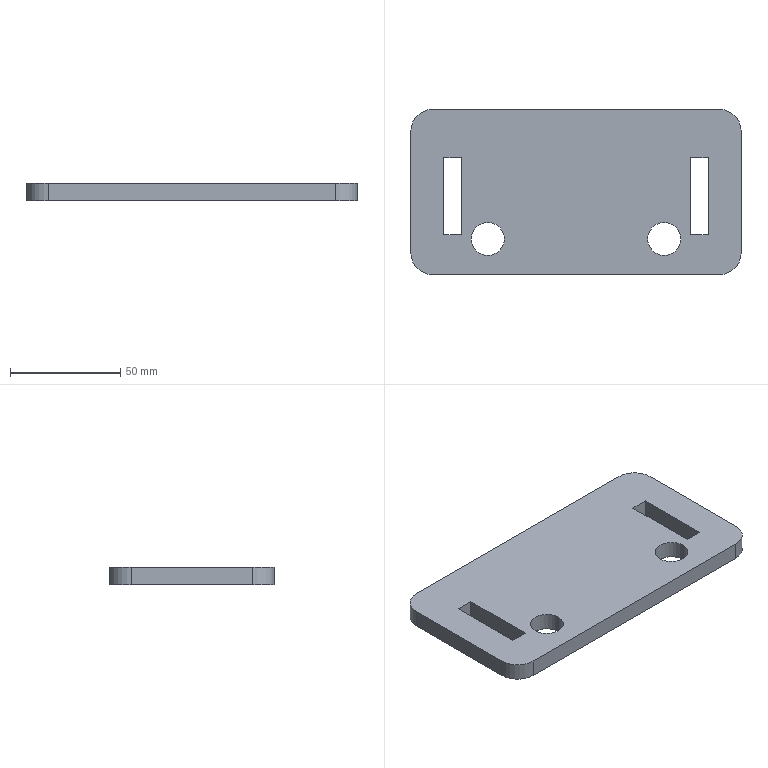Part | SolidWorks | features FlatPattern 1, SMBaseFlange 1, SheetMetal 1 | 1 solid | 22 faces | box 150 x 75 x 8 mm | volume 82006 mm3 | plane 14 | cylinder 8 | commonest cylinder face diameters 15 x4 20 x4
STEP:
#1=CARTESIAN_POINT('',(-47.5,148.277,8.));
#2=VERTEX_POINT('',#1);
#3=CARTESIAN_POINT('',(-32.5,148.277,8.));
#4=VERTEX_POINT('',#3);
#5=CARTESIAN_POINT('',(-40.,148.277,8.));
#6=DIRECTION('',(0.,0.,1.));
#7=DIRECTION('',(1.,0.,0.));
#8=AXIS2_PLACEMENT_3D('',#5,#6,#7);
#9=CIRCLE('',#8,7.5);
#10=EDGE_CURVE('',#2,#4,#9,.T.);
#11=ORIENTED_EDGE('',*,*,#10,.T.);
#12=CARTESIAN_POINT('',(-32.5,148.277,0.));
#13=VERTEX_POINT('',#12);
#14=CARTESIAN_POINT('',(-32.5,148.277,8.));
#15=DIRECTION('',(0.,0.,-1.));
#16=VECTOR('',#15,1000.);
#17=LINE('',#14,#16);
#18=EDGE_CURVE('',#4,#13,#17,.T.);
#19=ORIENTED_EDGE('',*,*,#18,.T.);
#20=CARTESIAN_POINT('',(-47.5,148.277,0.));
#21=VERTEX_POINT('',#20);
#22=CARTESIAN_POINT('',(-40.,148.277,0.));
#23=DIRECTION('',(0.,0.,1.));
#24=DIRECTION('',(1.,0.,0.));
#25=AXIS2_PLACEMENT_3D('',#22,#23,#24);
#26=CIRCLE('',#25,7.5);
#27=EDGE_CURVE('',#21,#13,#26,.T.);
#28=ORIENTED_EDGE('',*,*,#27,.F.);
#29=CARTESIAN_POINT('',(-47.5,148.277,8.));
#30=DIRECTION('',(0.,0.,-1.));
#31=VECTOR('',#30,1000.);
#32=LINE('',#29,#31);
#33=EDGE_CURVE('',#2,#21,#32,.T.);
#34=ORIENTED_EDGE('',*,*,#33,.F.);
#35=EDGE_LOOP('',(#11,#19,#28,#34));
#36=FACE_OUTER_BOUND('',#35,.T.);
#37=CARTESIAN_POINT('',(-40.,148.277,8.));
#38=DIRECTION('',(0.,0.,-1.));
#39=DIRECTION('',(-1.,0.,0.));
#40=AXIS2_PLACEMENT_3D('',#37,#38,#39);
#41=CYLINDRICAL_SURFACE('',#40,7.5);
#42=ADVANCED_FACE('',(#36),#41,.F.);
#43=CARTESIAN_POINT('',(32.5,148.277,8.));
#44=VERTEX_POINT('',#43);
#45=CARTESIAN_POINT('',(47.5,148.277,8.));
#46=VERTEX_POINT('',#45);
#47=CARTESIAN_POINT('',(40.,148.277,8.));
#48=DIRECTION('',(0.,0.,1.));
#49=DIRECTION('',(1.,0.,0.));
#50=AXIS2_PLACEMENT_3D('',#47,#48,#49);
#51=CIRCLE('',#50,7.5);
#52=EDGE_CURVE('',#44,#46,#51,.T.);
#53=ORIENTED_EDGE('',*,*,#52,.T.);
#54=CARTESIAN_POINT('',(47.5,148.277,0.));
#55=VERTEX_POINT('',#54);
#56=CARTESIAN_POINT('',(47.5,148.277,8.));
#57=DIRECTION('',(0.,0.,-1.));
#58=VECTOR('',#57,1000.);
#59=LINE('',#56,#58);
#60=EDGE_CURVE('',#46,#55,#59,.T.);
#61=ORIENTED_EDGE('',*,*,#60,.T.);
#62=CARTESIAN_POINT('',(32.5,148.277,0.));
#63=VERTEX_POINT('',#62);
#64=CARTESIAN_POINT('',(40.,148.277,0.));
#65=DIRECTION('',(0.,0.,1.));
#66=DIRECTION('',(1.,0.,0.));
#67=AXIS2_PLACEMENT_3D('',#64,#65,#66);
#68=CIRCLE('',#67,7.5);
#69=EDGE_CURVE('',#63,#55,#68,.T.);
#70=ORIENTED_EDGE('',*,*,#69,.F.);
#71=CARTESIAN_POINT('',(32.5,148.277,8.));
#72=DIRECTION('',(0.,0.,-1.));
#73=VECTOR('',#72,1000.);
#74=LINE('',#71,#73);
#75=EDGE_CURVE('',#44,#63,#74,.T.);
#76=ORIENTED_EDGE('',*,*,#75,.F.);
#77=EDGE_LOOP('',(#53,#61,#70,#76));
#78=FACE_OUTER_BOUND('',#77,.T.);
#79=CARTESIAN_POINT('',(40.,148.277,8.));
#80=DIRECTION('',(0.,0.,-1.));
#81=DIRECTION('',(-1.,0.,0.));
#82=AXIS2_PLACEMENT_3D('',#79,#80,#81);
#83=CYLINDRICAL_SURFACE('',#82,7.5);
#84=ADVANCED_FACE('',(#78),#83,.F.);
#85=ORIENTED_EDGE('',*,*,#52,.F.);
#86=CARTESIAN_POINT('',(40.,148.277,8.));
#87=DIRECTION('',(0.,0.,1.));
#88=DIRECTION('',(1.,0.,0.));
#89=AXIS2_PLACEMENT_3D('',#86,#87,#88);
#90=CIRCLE('',#89,7.5);
#91=EDGE_CURVE('',#46,#44,#90,.T.);
#92=ORIENTED_EDGE('',*,*,#91,.F.);
#93=EDGE_LOOP('',(#85,#92));
#94=FACE_BOUND('',#93,.T.);
#95=CARTESIAN_POINT('',(65.,132.079,8.));
#96=VERTEX_POINT('',#95);
#97=CARTESIAN_POINT('',(75.,142.079,8.));
#98=VERTEX_POINT('',#97);
#99=CARTESIAN_POINT('',(65.,142.079,8.));
#100=DIRECTION('',(0.,0.,1.));
#101=DIRECTION('',(1.,0.,0.));
#102=AXIS2_PLACEMENT_3D('',#99,#100,#101);
#103=CIRCLE('',#102,10.);
#104=EDGE_CURVE('',#96,#98,#103,.T.);
#105=ORIENTED_EDGE('',*,*,#104,.T.);
#106=CARTESIAN_POINT('',(75.,197.079,8.));
#107=VERTEX_POINT('',#106);
#108=CARTESIAN_POINT('',(75.,142.079,8.));
#109=DIRECTION('',(0.,1.,0.));
#110=VECTOR('',#109,1000.);
#111=LINE('',#108,#110);
#112=EDGE_CURVE('',#98,#107,#111,.T.);
#113=ORIENTED_EDGE('',*,*,#112,.T.);
#114=CARTESIAN_POINT('',(65.,207.079,8.));
#115=VERTEX_POINT('',#114);
#116=CARTESIAN_POINT('',(65.,197.079,8.));
#117=DIRECTION('',(0.,0.,1.));
#118=DIRECTION('',(1.,0.,0.));
#119=AXIS2_PLACEMENT_3D('',#116,#117,#118);
#120=CIRCLE('',#119,10.);
#121=EDGE_CURVE('',#107,#115,#120,.T.);
#122=ORIENTED_EDGE('',*,*,#121,.T.);
#123=CARTESIAN_POINT('',(-65.,207.079,8.));
#124=VERTEX_POINT('',#123);
#125=CARTESIAN_POINT('',(65.,207.079,8.));
#126=DIRECTION('',(-1.,0.,0.));
#127=VECTOR('',#126,1000.);
#128=LINE('',#125,#127);
#129=EDGE_CURVE('',#115,#124,#128,.T.);
#130=ORIENTED_EDGE('',*,*,#129,.T.);
#131=CARTESIAN_POINT('',(-75.,197.079,8.));
#132=VERTEX_POINT('',#131);
#133=CARTESIAN_POINT('',(-65.,197.079,8.));
#134=DIRECTION('',(0.,0.,1.));
#135=DIRECTION('',(1.,0.,0.));
#136=AXIS2_PLACEMENT_3D('',#133,#134,#135);
#137=CIRCLE('',#136,10.);
#138=EDGE_CURVE('',#124,#132,#137,.T.);
#139=ORIENTED_EDGE('',*,*,#138,.T.);
#140=CARTESIAN_POINT('',(-75.,142.079,8.));
#141=VERTEX_POINT('',#140);
#142=CARTESIAN_POINT('',(-75.,197.079,8.));
#143=DIRECTION('',(0.,-1.,0.));
#144=VECTOR('',#143,1000.);
#145=LINE('',#142,#144);
#146=EDGE_CURVE('',#132,#141,#145,.T.);
#147=ORIENTED_EDGE('',*,*,#146,.T.);
#148=CARTESIAN_POINT('',(-65.,132.079,8.));
#149=VERTEX_POINT('',#148);
#150=CARTESIAN_POINT('',(-65.,142.079,8.));
#151=DIRECTION('',(0.,0.,1.));
#152=DIRECTION('',(-1.,0.,0.));
#153=AXIS2_PLACEMENT_3D('',#150,#151,#152);
#154=CIRCLE('',#153,10.);
#155=EDGE_CURVE('',#141,#149,#154,.T.);
#156=ORIENTED_EDGE('',*,*,#155,.T.);
#157=CARTESIAN_POINT('',(-65.,132.079,8.));
#158=DIRECTION('',(1.,0.,0.));
#159=VECTOR('',#158,1000.);
#160=LINE('',#157,#159);
#161=EDGE_CURVE('',#149,#96,#160,.T.);
#162=ORIENTED_EDGE('',*,*,#161,.T.);
#163=EDGE_LOOP('',(#105,#113,#122,#130,#139,#147,#156,#162));
#164=FACE_OUTER_BOUND('',#163,.T.);
#165=ORIENTED_EDGE('',*,*,#10,.F.);
#166=CARTESIAN_POINT('',(-40.,148.277,8.));
#167=DIRECTION('',(0.,0.,1.));
#168=DIRECTION('',(1.,0.,0.));
#169=AXIS2_PLACEMENT_3D('',#166,#167,#168);
#170=CIRCLE('',#169,7.5);
#171=EDGE_CURVE('',#4,#2,#170,.T.);
#172=ORIENTED_EDGE('',*,*,#171,.F.);
#173=EDGE_LOOP('',(#165,#172));
#174=FACE_BOUND('',#173,.T.);
#175=CARTESIAN_POINT('',(60.,185.084,8.));
#176=VERTEX_POINT('',#175);
#177=CARTESIAN_POINT('',(52.,185.084,8.));
#178=VERTEX_POINT('',#177);
#179=CARTESIAN_POINT('',(60.,185.084,8.));
#180=DIRECTION('',(-1.,0.,0.));
#181=VECTOR('',#180,1000.);
#182=LINE('',#179,#181);
#183=EDGE_CURVE('',#176,#178,#182,.T.);
#184=ORIENTED_EDGE('',*,*,#183,.F.);
#185=CARTESIAN_POINT('',(60.,150.084,8.));
#186=VERTEX_POINT('',#185);
#187=CARTESIAN_POINT('',(60.,185.084,8.));
#188=DIRECTION('',(0.,1.,0.));
#189=VECTOR('',#188,1000.);
#190=LINE('',#187,#189);
#191=EDGE_CURVE('',#186,#176,#190,.T.);
#192=ORIENTED_EDGE('',*,*,#191,.F.);
#193=CARTESIAN_POINT('',(52.,150.084,8.));
#194=VERTEX_POINT('',#193);
#195=CARTESIAN_POINT('',(60.,150.084,8.));
#196=DIRECTION('',(1.,0.,0.));
#197=VECTOR('',#196,1000.);
#198=LINE('',#195,#197);
#199=EDGE_CURVE('',#194,#186,#198,.T.);
#200=ORIENTED_EDGE('',*,*,#199,.F.);
#201=CARTESIAN_POINT('',(52.,185.084,8.));
#202=DIRECTION('',(0.,-1.,0.));
#203=VECTOR('',#202,1000.);
#204=LINE('',#201,#203);
#205=EDGE_CURVE('',#178,#194,#204,.T.);
#206=ORIENTED_EDGE('',*,*,#205,.F.);
#207=EDGE_LOOP('',(#184,#192,#200,#206));
#208=FACE_BOUND('',#207,.T.);
#209=CARTESIAN_POINT('',(-52.,185.084,8.));
#210=VERTEX_POINT('',#209);
#211=CARTESIAN_POINT('',(-60.,185.084,8.));
#212=VERTEX_POINT('',#211);
#213=CARTESIAN_POINT('',(-52.,185.084,8.));
#214=DIRECTION('',(-1.,0.,0.));
#215=VECTOR('',#214,1000.);
#216=LINE('',#213,#215);
#217=EDGE_CURVE('',#210,#212,#216,.T.);
#218=ORIENTED_EDGE('',*,*,#217,.F.);
#219=CARTESIAN_POINT('',(-52.,150.084,8.));
#220=VERTEX_POINT('',#219);
#221=CARTESIAN_POINT('',(-52.,185.084,8.));
#222=DIRECTION('',(0.,1.,0.));
#223=VECTOR('',#222,1000.);
#224=LINE('',#221,#223);
#225=EDGE_CURVE('',#220,#210,#224,.T.);
#226=ORIENTED_EDGE('',*,*,#225,.F.);
#227=CARTESIAN_POINT('',(-60.,150.084,8.));
#228=VERTEX_POINT('',#227);
#229=CARTESIAN_POINT('',(-52.,150.084,8.));
#230=DIRECTION('',(1.,0.,0.));
#231=VECTOR('',#230,1000.);
#232=LINE('',#229,#231);
#233=EDGE_CURVE('',#228,#220,#232,.T.);
#234=ORIENTED_EDGE('',*,*,#233,.F.);
#235=CARTESIAN_POINT('',(-60.,185.084,8.));
#236=DIRECTION('',(0.,-1.,0.));
#237=VECTOR('',#236,1000.);
#238=LINE('',#235,#237);
#239=EDGE_CURVE('',#212,#228,#238,.T.);
#240=ORIENTED_EDGE('',*,*,#239,.F.);
#241=EDGE_LOOP('',(#218,#226,#234,#240));
#242=FACE_BOUND('',#241,.T.);
#243=CARTESIAN_POINT('',(65.,142.079,8.));
#244=DIRECTION('',(0.,0.,1.));
#245=DIRECTION('',(1.,0.,0.));
#246=AXIS2_PLACEMENT_3D('',#243,#244,#245);
#247=PLANE('',#246);
#248=ADVANCED_FACE('',(#94,#164,#174,#208,#242),#247,.T.);
#249=CARTESIAN_POINT('',(60.,150.084,0.));
#250=VERTEX_POINT('',#249);
#251=CARTESIAN_POINT('',(60.,185.084,0.));
#252=VERTEX_POINT('',#251);
#253=CARTESIAN_POINT('',(60.,185.084,0.));
#254=DIRECTION('',(0.,1.,0.));
#255=VECTOR('',#254,1000.);
#256=LINE('',#253,#255);
#257=EDGE_CURVE('',#250,#252,#256,.T.);
#258=ORIENTED_EDGE('',*,*,#257,.T.);
#259=CARTESIAN_POINT('',(52.,185.084,0.));
#260=VERTEX_POINT('',#259);
#261=CARTESIAN_POINT('',(60.,185.084,0.));
#262=DIRECTION('',(-1.,0.,0.));
#263=VECTOR('',#262,1000.);
#264=LINE('',#261,#263);
#265=EDGE_CURVE('',#252,#260,#264,.T.);
#266=ORIENTED_EDGE('',*,*,#265,.T.);
#267=CARTESIAN_POINT('',(52.,150.084,0.));
#268=VERTEX_POINT('',#267);
#269=CARTESIAN_POINT('',(52.,185.084,0.));
#270=DIRECTION('',(0.,-1.,0.));
#271=VECTOR('',#270,1000.);
#272=LINE('',#269,#271);
#273=EDGE_CURVE('',#260,#268,#272,.T.);
#274=ORIENTED_EDGE('',*,*,#273,.T.);
#275=CARTESIAN_POINT('',(60.,150.084,0.));
#276=DIRECTION('',(1.,0.,0.));
#277=VECTOR('',#276,1000.);
#278=LINE('',#275,#277);
#279=EDGE_CURVE('',#268,#250,#278,.T.);
#280=ORIENTED_EDGE('',*,*,#279,.T.);
#281=EDGE_LOOP('',(#258,#266,#274,#280));
#282=FACE_BOUND('',#281,.T.);
#283=CARTESIAN_POINT('',(65.,132.079,0.));
#284=VERTEX_POINT('',#283);
#285=CARTESIAN_POINT('',(75.,142.079,0.));
#286=VERTEX_POINT('',#285);
#287=CARTESIAN_POINT('',(65.,142.079,0.));
#288=DIRECTION('',(0.,0.,1.));
#289=DIRECTION('',(1.,0.,0.));
#290=AXIS2_PLACEMENT_3D('',#287,#288,#289);
#291=CIRCLE('',#290,10.);
#292=EDGE_CURVE('',#284,#286,#291,.T.);
#293=ORIENTED_EDGE('',*,*,#292,.F.);
#294=CARTESIAN_POINT('',(-65.,132.079,0.));
#295=VERTEX_POINT('',#294);
#296=CARTESIAN_POINT('',(-65.,132.079,0.));
#297=DIRECTION('',(1.,0.,0.));
#298=VECTOR('',#297,1000.);
#299=LINE('',#296,#298);
#300=EDGE_CURVE('',#295,#284,#299,.T.);
#301=ORIENTED_EDGE('',*,*,#300,.F.);
#302=CARTESIAN_POINT('',(-75.,142.079,0.));
#303=VERTEX_POINT('',#302);
#304=CARTESIAN_POINT('',(-65.,142.079,0.));
#305=DIRECTION('',(0.,0.,1.));
#306=DIRECTION('',(-1.,0.,0.));
#307=AXIS2_PLACEMENT_3D('',#304,#305,#306);
#308=CIRCLE('',#307,10.);
#309=EDGE_CURVE('',#303,#295,#308,.T.);
#310=ORIENTED_EDGE('',*,*,#309,.F.);
#311=CARTESIAN_POINT('',(-75.,197.079,0.));
#312=VERTEX_POINT('',#311);
#313=CARTESIAN_POINT('',(-75.,197.079,0.));
#314=DIRECTION('',(0.,-1.,0.));
#315=VECTOR('',#314,1000.);
#316=LINE('',#313,#315);
#317=EDGE_CURVE('',#312,#303,#316,.T.);
#318=ORIENTED_EDGE('',*,*,#317,.F.);
#319=CARTESIAN_POINT('',(-65.,207.079,0.));
#320=VERTEX_POINT('',#319);
#321=CARTESIAN_POINT('',(-65.,197.079,0.));
#322=DIRECTION('',(0.,0.,1.));
#323=DIRECTION('',(1.,0.,0.));
#324=AXIS2_PLACEMENT_3D('',#321,#322,#323);
#325=CIRCLE('',#324,10.);
#326=EDGE_CURVE('',#320,#312,#325,.T.);
#327=ORIENTED_EDGE('',*,*,#326,.F.);
#328=CARTESIAN_POINT('',(65.,207.079,0.));
#329=VERTEX_POINT('',#328);
#330=CARTESIAN_POINT('',(65.,207.079,0.));
#331=DIRECTION('',(-1.,0.,0.));
#332=VECTOR('',#331,1000.);
#333=LINE('',#330,#332);
#334=EDGE_CURVE('',#329,#320,#333,.T.);
#335=ORIENTED_EDGE('',*,*,#334,.F.);
#336=CARTESIAN_POINT('',(75.,197.079,0.));
#337=VERTEX_POINT('',#336);
#338=CARTESIAN_POINT('',(65.,197.079,0.));
#339=DIRECTION('',(0.,0.,1.));
#340=DIRECTION('',(1.,0.,0.));
#341=AXIS2_PLACEMENT_3D('',#338,#339,#340);
#342=CIRCLE('',#341,10.);
#343=EDGE_CURVE('',#337,#329,#342,.T.);
#344=ORIENTED_EDGE('',*,*,#343,.F.);
#345=CARTESIAN_POINT('',(75.,142.079,0.));
#346=DIRECTION('',(0.,1.,0.));
#347=VECTOR('',#346,1000.);
#348=LINE('',#345,#347);
#349=EDGE_CURVE('',#286,#337,#348,.T.);
#350=ORIENTED_EDGE('',*,*,#349,.F.);
#351=EDGE_LOOP('',(#293,#301,#310,#318,#327,#335,#344,#350));
#352=FACE_OUTER_BOUND('',#351,.T.);
#353=ORIENTED_EDGE('',*,*,#69,.T.);
#354=CARTESIAN_POINT('',(40.,148.277,0.));
#355=DIRECTION('',(0.,0.,1.));
#356=DIRECTION('',(1.,0.,0.));
#357=AXIS2_PLACEMENT_3D('',#354,#355,#356);
#358=CIRCLE('',#357,7.5);
#359=EDGE_CURVE('',#55,#63,#358,.T.);
#360=ORIENTED_EDGE('',*,*,#359,.T.);
#361=EDGE_LOOP('',(#353,#360));
#362=FACE_BOUND('',#361,.T.);
#363=ORIENTED_EDGE('',*,*,#27,.T.);
#364=CARTESIAN_POINT('',(-40.,148.277,0.));
#365=DIRECTION('',(0.,0.,1.));
#366=DIRECTION('',(1.,0.,0.));
#367=AXIS2_PLACEMENT_3D('',#364,#365,#366);
#368=CIRCLE('',#367,7.5);
#369=EDGE_CURVE('',#13,#21,#368,.T.);
#370=ORIENTED_EDGE('',*,*,#369,.T.);
#371=EDGE_LOOP('',(#363,#370));
#372=FACE_BOUND('',#371,.T.);
#373=CARTESIAN_POINT('',(-52.,150.084,0.));
#374=VERTEX_POINT('',#373);
#375=CARTESIAN_POINT('',(-52.,185.084,0.));
#376=VERTEX_POINT('',#375);
#377=CARTESIAN_POINT('',(-52.,185.084,0.));
#378=DIRECTION('',(0.,1.,0.));
#379=VECTOR('',#378,1000.);
#380=LINE('',#377,#379);
#381=EDGE_CURVE('',#374,#376,#380,.T.);
#382=ORIENTED_EDGE('',*,*,#381,.T.);
#383=CARTESIAN_POINT('',(-60.,185.084,0.));
#384=VERTEX_POINT('',#383);
#385=CARTESIAN_POINT('',(-52.,185.084,0.));
#386=DIRECTION('',(-1.,0.,0.));
#387=VECTOR('',#386,1000.);
#388=LINE('',#385,#387);
#389=EDGE_CURVE('',#376,#384,#388,.T.);
#390=ORIENTED_EDGE('',*,*,#389,.T.);
#391=CARTESIAN_POINT('',(-60.,150.084,0.));
#392=VERTEX_POINT('',#391);
#393=CARTESIAN_POINT('',(-60.,185.084,0.));
#394=DIRECTION('',(0.,-1.,0.));
#395=VECTOR('',#394,1000.);
#396=LINE('',#393,#395);
#397=EDGE_CURVE('',#384,#392,#396,.T.);
#398=ORIENTED_EDGE('',*,*,#397,.T.);
#399=CARTESIAN_POINT('',(-52.,150.084,0.));
#400=DIRECTION('',(1.,0.,0.));
#401=VECTOR('',#400,1000.);
#402=LINE('',#399,#401);
#403=EDGE_CURVE('',#392,#374,#402,.T.);
#404=ORIENTED_EDGE('',*,*,#403,.T.);
#405=EDGE_LOOP('',(#382,#390,#398,#404));
#406=FACE_BOUND('',#405,.T.);
#407=CARTESIAN_POINT('',(65.,142.079,0.));
#408=DIRECTION('',(0.,0.,1.));
#409=DIRECTION('',(1.,0.,0.));
#410=AXIS2_PLACEMENT_3D('',#407,#408,#409);
#411=PLANE('',#410);
#412=ADVANCED_FACE('',(#282,#352,#362,#372,#406),#411,.F.);
#413=ORIENTED_EDGE('',*,*,#292,.T.);
#414=CARTESIAN_POINT('',(75.,142.079,8.));
#415=DIRECTION('',(0.,0.,-1.));
#416=VECTOR('',#415,1000.);
#417=LINE('',#414,#416);
#418=EDGE_CURVE('',#98,#286,#417,.T.);
#419=ORIENTED_EDGE('',*,*,#418,.F.);
#420=ORIENTED_EDGE('',*,*,#104,.F.);
#421=CARTESIAN_POINT('',(65.,132.079,8.));
#422=DIRECTION('',(0.,0.,-1.));
#423=VECTOR('',#422,1000.);
#424=LINE('',#421,#423);
#425=EDGE_CURVE('',#96,#284,#424,.T.);
#426=ORIENTED_EDGE('',*,*,#425,.T.);
#427=EDGE_LOOP('',(#413,#419,#420,#426));
#428=FACE_OUTER_BOUND('',#427,.T.);
#429=CARTESIAN_POINT('',(65.,142.079,8.));
#430=DIRECTION('',(0.,0.,-1.));
#431=DIRECTION('',(-1.,0.,0.));
#432=AXIS2_PLACEMENT_3D('',#429,#430,#431);
#433=CYLINDRICAL_SURFACE('',#432,10.);
#434=ADVANCED_FACE('',(#428),#433,.T.);
#435=ORIENTED_EDGE('',*,*,#349,.T.);
#436=CARTESIAN_POINT('',(75.,197.079,8.));
#437=DIRECTION('',(0.,0.,-1.));
#438=VECTOR('',#437,1000.);
#439=LINE('',#436,#438);
#440=EDGE_CURVE('',#107,#337,#439,.T.);
#441=ORIENTED_EDGE('',*,*,#440,.F.);
#442=ORIENTED_EDGE('',*,*,#112,.F.);
#443=ORIENTED_EDGE('',*,*,#418,.T.);
#444=EDGE_LOOP('',(#435,#441,#442,#443));
#445=FACE_OUTER_BOUND('',#444,.T.);
#446=CARTESIAN_POINT('',(75.,142.079,8.));
#447=DIRECTION('',(-1.,0.,0.));
#448=DIRECTION('',(0.,-1.,0.));
#449=AXIS2_PLACEMENT_3D('',#446,#447,#448);
#450=PLANE('',#449);
#451=ADVANCED_FACE('',(#445),#450,.F.);
#452=ORIENTED_EDGE('',*,*,#343,.T.);
#453=CARTESIAN_POINT('',(65.,207.079,8.));
#454=DIRECTION('',(0.,0.,-1.));
#455=VECTOR('',#454,1000.);
#456=LINE('',#453,#455);
#457=EDGE_CURVE('',#115,#329,#456,.T.);
#458=ORIENTED_EDGE('',*,*,#457,.F.);
#459=ORIENTED_EDGE('',*,*,#121,.F.);
#460=ORIENTED_EDGE('',*,*,#440,.T.);
#461=EDGE_LOOP('',(#452,#458,#459,#460));
#462=FACE_OUTER_BOUND('',#461,.T.);
#463=CARTESIAN_POINT('',(65.,197.079,8.));
#464=DIRECTION('',(0.,0.,-1.));
#465=DIRECTION('',(-1.,0.,0.));
#466=AXIS2_PLACEMENT_3D('',#463,#464,#465);
#467=CYLINDRICAL_SURFACE('',#466,10.);
#468=ADVANCED_FACE('',(#462),#467,.T.);
#469=ORIENTED_EDGE('',*,*,#334,.T.);
#470=CARTESIAN_POINT('',(-65.,207.079,8.));
#471=DIRECTION('',(0.,0.,-1.));
#472=VECTOR('',#471,1000.);
#473=LINE('',#470,#472);
#474=EDGE_CURVE('',#124,#320,#473,.T.);
#475=ORIENTED_EDGE('',*,*,#474,.F.);
#476=ORIENTED_EDGE('',*,*,#129,.F.);
#477=ORIENTED_EDGE('',*,*,#457,.T.);
#478=EDGE_LOOP('',(#469,#475,#476,#477));
#479=FACE_OUTER_BOUND('',#478,.T.);
#480=CARTESIAN_POINT('',(65.,207.079,8.));
#481=DIRECTION('',(0.,-1.,0.));
#482=DIRECTION('',(1.,0.,0.));
#483=AXIS2_PLACEMENT_3D('',#480,#481,#482);
#484=PLANE('',#483);
#485=ADVANCED_FACE('',(#479),#484,.F.);
#486=ORIENTED_EDGE('',*,*,#326,.T.);
#487=CARTESIAN_POINT('',(-75.,197.079,8.));
#488=DIRECTION('',(0.,0.,-1.));
#489=VECTOR('',#488,1000.);
#490=LINE('',#487,#489);
#491=EDGE_CURVE('',#132,#312,#490,.T.);
#492=ORIENTED_EDGE('',*,*,#491,.F.);
#493=ORIENTED_EDGE('',*,*,#138,.F.);
#494=ORIENTED_EDGE('',*,*,#474,.T.);
#495=EDGE_LOOP('',(#486,#492,#493,#494));
#496=FACE_OUTER_BOUND('',#495,.T.);
#497=CARTESIAN_POINT('',(-65.,197.079,8.));
#498=DIRECTION('',(0.,0.,-1.));
#499=DIRECTION('',(-1.,0.,0.));
#500=AXIS2_PLACEMENT_3D('',#497,#498,#499);
#501=CYLINDRICAL_SURFACE('',#500,10.);
#502=ADVANCED_FACE('',(#496),#501,.T.);
#503=ORIENTED_EDGE('',*,*,#317,.T.);
#504=CARTESIAN_POINT('',(-75.,142.079,8.));
#505=DIRECTION('',(0.,0.,-1.));
#506=VECTOR('',#505,1000.);
#507=LINE('',#504,#506);
#508=EDGE_CURVE('',#141,#303,#507,.T.);
#509=ORIENTED_EDGE('',*,*,#508,.F.);
#510=ORIENTED_EDGE('',*,*,#146,.F.);
#511=ORIENTED_EDGE('',*,*,#491,.T.);
#512=EDGE_LOOP('',(#503,#509,#510,#511));
#513=FACE_OUTER_BOUND('',#512,.T.);
#514=CARTESIAN_POINT('',(-75.,197.079,8.));
#515=DIRECTION('',(1.,0.,0.));
#516=DIRECTION('',(0.,1.,0.));
#517=AXIS2_PLACEMENT_3D('',#514,#515,#516);
#518=PLANE('',#517);
#519=ADVANCED_FACE('',(#513),#518,.F.);
#520=ORIENTED_EDGE('',*,*,#309,.T.);
#521=CARTESIAN_POINT('',(-65.,132.079,8.));
#522=DIRECTION('',(0.,0.,-1.));
#523=VECTOR('',#522,1000.);
#524=LINE('',#521,#523);
#525=EDGE_CURVE('',#149,#295,#524,.T.);
#526=ORIENTED_EDGE('',*,*,#525,.F.);
#527=ORIENTED_EDGE('',*,*,#155,.F.);
#528=ORIENTED_EDGE('',*,*,#508,.T.);
#529=EDGE_LOOP('',(#520,#526,#527,#528));
#530=FACE_OUTER_BOUND('',#529,.T.);
#531=CARTESIAN_POINT('',(-65.,142.079,8.));
#532=DIRECTION('',(0.,0.,-1.));
#533=DIRECTION('',(-1.,0.,0.));
#534=AXIS2_PLACEMENT_3D('',#531,#532,#533);
#535=CYLINDRICAL_SURFACE('',#534,10.);
#536=ADVANCED_FACE('',(#530),#535,.T.);
#537=ORIENTED_EDGE('',*,*,#300,.T.);
#538=ORIENTED_EDGE('',*,*,#425,.F.);
#539=ORIENTED_EDGE('',*,*,#161,.F.);
#540=ORIENTED_EDGE('',*,*,#525,.T.);
#541=EDGE_LOOP('',(#537,#538,#539,#540));
#542=FACE_OUTER_BOUND('',#541,.T.);
#543=CARTESIAN_POINT('',(-65.,132.079,8.));
#544=DIRECTION('',(0.,1.,0.));
#545=DIRECTION('',(0.,0.,1.));
#546=AXIS2_PLACEMENT_3D('',#543,#544,#545);
#547=PLANE('',#546);
#548=ADVANCED_FACE('',(#542),#547,.F.);
#549=ORIENTED_EDGE('',*,*,#60,.F.);
#550=ORIENTED_EDGE('',*,*,#91,.T.);
#551=ORIENTED_EDGE('',*,*,#75,.T.);
#552=ORIENTED_EDGE('',*,*,#359,.F.);
#553=EDGE_LOOP('',(#549,#550,#551,#552));
#554=FACE_OUTER_BOUND('',#553,.T.);
#555=CARTESIAN_POINT('',(40.,148.277,8.));
#556=DIRECTION('',(0.,0.,-1.));
#557=DIRECTION('',(-1.,0.,0.));
#558=AXIS2_PLACEMENT_3D('',#555,#556,#557);
#559=CYLINDRICAL_SURFACE('',#558,7.5);
#560=ADVANCED_FACE('',(#554),#559,.F.);
#561=ORIENTED_EDGE('',*,*,#18,.F.);
#562=ORIENTED_EDGE('',*,*,#171,.T.);
#563=ORIENTED_EDGE('',*,*,#33,.T.);
#564=ORIENTED_EDGE('',*,*,#369,.F.);
#565=EDGE_LOOP('',(#561,#562,#563,#564));
#566=FACE_OUTER_BOUND('',#565,.T.);
#567=CARTESIAN_POINT('',(-40.,148.277,8.));
#568=DIRECTION('',(0.,0.,-1.));
#569=DIRECTION('',(-1.,0.,0.));
#570=AXIS2_PLACEMENT_3D('',#567,#568,#569);
#571=CYLINDRICAL_SURFACE('',#570,7.5);
#572=ADVANCED_FACE('',(#566),#571,.F.);
#573=ORIENTED_EDGE('',*,*,#257,.F.);
#574=CARTESIAN_POINT('',(60.,150.084,8.));
#575=DIRECTION('',(0.,0.,-1.));
#576=VECTOR('',#575,1000.);
#577=LINE('',#574,#576);
#578=EDGE_CURVE('',#186,#250,#577,.T.);
#579=ORIENTED_EDGE('',*,*,#578,.F.);
#580=ORIENTED_EDGE('',*,*,#191,.T.);
#581=CARTESIAN_POINT('',(60.,185.084,8.));
#582=DIRECTION('',(0.,0.,-1.));
#583=VECTOR('',#582,1000.);
#584=LINE('',#581,#583);
#585=EDGE_CURVE('',#176,#252,#584,.T.);
#586=ORIENTED_EDGE('',*,*,#585,.T.);
#587=EDGE_LOOP('',(#573,#579,#580,#586));
#588=FACE_OUTER_BOUND('',#587,.T.);
#589=CARTESIAN_POINT('',(60.,185.084,8.));
#590=DIRECTION('',(-1.,0.,0.));
#591=DIRECTION('',(0.,0.,1.));
#592=AXIS2_PLACEMENT_3D('',#589,#590,#591);
#593=PLANE('',#592);
#594=ADVANCED_FACE('',(#588),#593,.T.);
#595=ORIENTED_EDGE('',*,*,#265,.F.);
#596=ORIENTED_EDGE('',*,*,#585,.F.);
#597=ORIENTED_EDGE('',*,*,#183,.T.);
#598=CARTESIAN_POINT('',(52.,185.084,8.));
#599=DIRECTION('',(0.,0.,-1.));
#600=VECTOR('',#599,1000.);
#601=LINE('',#598,#600);
#602=EDGE_CURVE('',#178,#260,#601,.T.);
#603=ORIENTED_EDGE('',*,*,#602,.T.);
#604=EDGE_LOOP('',(#595,#596,#597,#603));
#605=FACE_OUTER_BOUND('',#604,.T.);
#606=CARTESIAN_POINT('',(60.,185.084,8.));
#607=DIRECTION('',(0.,-1.,0.));
#608=DIRECTION('',(0.,0.,-1.));
#609=AXIS2_PLACEMENT_3D('',#606,#607,#608);
#610=PLANE('',#609);
#611=ADVANCED_FACE('',(#605),#610,.T.);
#612=ORIENTED_EDGE('',*,*,#273,.F.);
#613=ORIENTED_EDGE('',*,*,#602,.F.);
#614=ORIENTED_EDGE('',*,*,#205,.T.);
#615=CARTESIAN_POINT('',(52.,150.084,8.));
#616=DIRECTION('',(0.,0.,-1.));
#617=VECTOR('',#616,1000.);
#618=LINE('',#615,#617);
#619=EDGE_CURVE('',#194,#268,#618,.T.);
#620=ORIENTED_EDGE('',*,*,#619,.T.);
#621=EDGE_LOOP('',(#612,#613,#614,#620));
#622=FACE_OUTER_BOUND('',#621,.T.);
#623=CARTESIAN_POINT('',(52.,185.084,8.));
#624=DIRECTION('',(1.,0.,0.));
#625=DIRECTION('',(0.,0.,-1.));
#626=AXIS2_PLACEMENT_3D('',#623,#624,#625);
#627=PLANE('',#626);
#628=ADVANCED_FACE('',(#622),#627,.T.);
#629=ORIENTED_EDGE('',*,*,#279,.F.);
#630=ORIENTED_EDGE('',*,*,#619,.F.);
#631=ORIENTED_EDGE('',*,*,#199,.T.);
#632=ORIENTED_EDGE('',*,*,#578,.T.);
#633=EDGE_LOOP('',(#629,#630,#631,#632));
#634=FACE_OUTER_BOUND('',#633,.T.);
#635=CARTESIAN_POINT('',(60.,150.084,8.));
#636=DIRECTION('',(0.,1.,0.));
#637=DIRECTION('',(0.,0.,1.));
#638=AXIS2_PLACEMENT_3D('',#635,#636,#637);
#639=PLANE('',#638);
#640=ADVANCED_FACE('',(#634),#639,.T.);
#641=ORIENTED_EDGE('',*,*,#381,.F.);
#642=CARTESIAN_POINT('',(-52.,150.084,8.));
#643=DIRECTION('',(0.,0.,-1.));
#644=VECTOR('',#643,1000.);
#645=LINE('',#642,#644);
#646=EDGE_CURVE('',#220,#374,#645,.T.);
#647=ORIENTED_EDGE('',*,*,#646,.F.);
#648=ORIENTED_EDGE('',*,*,#225,.T.);
#649=CARTESIAN_POINT('',(-52.,185.084,8.));
#650=DIRECTION('',(0.,0.,-1.));
#651=VECTOR('',#650,1000.);
#652=LINE('',#649,#651);
#653=EDGE_CURVE('',#210,#376,#652,.T.);
#654=ORIENTED_EDGE('',*,*,#653,.T.);
#655=EDGE_LOOP('',(#641,#647,#648,#654));
#656=FACE_OUTER_BOUND('',#655,.T.);
#657=CARTESIAN_POINT('',(-52.,185.084,8.));
#658=DIRECTION('',(-1.,0.,0.));
#659=DIRECTION('',(0.,0.,1.));
#660=AXIS2_PLACEMENT_3D('',#657,#658,#659);
#661=PLANE('',#660);
#662=ADVANCED_FACE('',(#656),#661,.T.);
#663=ORIENTED_EDGE('',*,*,#389,.F.);
#664=ORIENTED_EDGE('',*,*,#653,.F.);
#665=ORIENTED_EDGE('',*,*,#217,.T.);
#666=CARTESIAN_POINT('',(-60.,185.084,8.));
#667=DIRECTION('',(0.,0.,-1.));
#668=VECTOR('',#667,1000.);
#669=LINE('',#666,#668);
#670=EDGE_CURVE('',#212,#384,#669,.T.);
#671=ORIENTED_EDGE('',*,*,#670,.T.);
#672=EDGE_LOOP('',(#663,#664,#665,#671));
#673=FACE_OUTER_BOUND('',#672,.T.);
#674=CARTESIAN_POINT('',(-52.,185.084,8.));
#675=DIRECTION('',(0.,-1.,0.));
#676=DIRECTION('',(0.,0.,-1.));
#677=AXIS2_PLACEMENT_3D('',#674,#675,#676);
#678=PLANE('',#677);
#679=ADVANCED_FACE('',(#673),#678,.T.);
#680=ORIENTED_EDGE('',*,*,#397,.F.);
#681=ORIENTED_EDGE('',*,*,#670,.F.);
#682=ORIENTED_EDGE('',*,*,#239,.T.);
#683=CARTESIAN_POINT('',(-60.,150.084,8.));
#684=DIRECTION('',(0.,0.,-1.));
#685=VECTOR('',#684,1000.);
#686=LINE('',#683,#685);
#687=EDGE_CURVE('',#228,#392,#686,.T.);
#688=ORIENTED_EDGE('',*,*,#687,.T.);
#689=EDGE_LOOP('',(#680,#681,#682,#688));
#690=FACE_OUTER_BOUND('',#689,.T.);
#691=CARTESIAN_POINT('',(-60.,185.084,8.));
#692=DIRECTION('',(1.,0.,0.));
#693=DIRECTION('',(0.,0.,-1.));
#694=AXIS2_PLACEMENT_3D('',#691,#692,#693);
#695=PLANE('',#694);
#696=ADVANCED_FACE('',(#690),#695,.T.);
#697=ORIENTED_EDGE('',*,*,#403,.F.);
#698=ORIENTED_EDGE('',*,*,#687,.F.);
#699=ORIENTED_EDGE('',*,*,#233,.T.);
#700=ORIENTED_EDGE('',*,*,#646,.T.);
#701=EDGE_LOOP('',(#697,#698,#699,#700));
#702=FACE_OUTER_BOUND('',#701,.T.);
#703=CARTESIAN_POINT('',(-52.,150.084,8.));
#704=DIRECTION('',(0.,1.,0.));
#705=DIRECTION('',(0.,0.,1.));
#706=AXIS2_PLACEMENT_3D('',#703,#704,#705);
#707=PLANE('',#706);
#708=ADVANCED_FACE('',(#702),#707,.T.);
#709=CLOSED_SHELL('',(#42,#84,#248,#412,#434,#451,#468,#485,#502,#519,#536,#548,#560,#572,#594,#611,#628,#640,#662,#679,#696,#708));
#710=MANIFOLD_SOLID_BREP('',#709);
#711=CARTESIAN_POINT('',(0.,0.,0.));
#712=DIRECTION('',(0.,0.,1.));
#713=DIRECTION('',(1.,0.,0.));
#714=AXIS2_PLACEMENT_3D('',#711,#712,#713);
#715=(LENGTH_UNIT()NAMED_UNIT(*)SI_UNIT(.MILLI.,.METRE.));
#716=UNCERTAINTY_MEASURE_WITH_UNIT(LENGTH_MEASURE(0.00001),#715,'','');
#717=(NAMED_UNIT(*)PLANE_ANGLE_UNIT()SI_UNIT($,.RADIAN.));
#718=(NAMED_UNIT(*)SI_UNIT($,.STERADIAN.)SOLID_ANGLE_UNIT());
#719=(GEOMETRIC_REPRESENTATION_CONTEXT(3)GLOBAL_UNCERTAINTY_ASSIGNED_CONTEXT((#716))GLOBAL_UNIT_ASSIGNED_CONTEXT((#715,#717,#718))REPRESENTATION_CONTEXT('',''));
#720=ADVANCED_BREP_SHAPE_REPRESENTATION('',(#710,#714),#719);